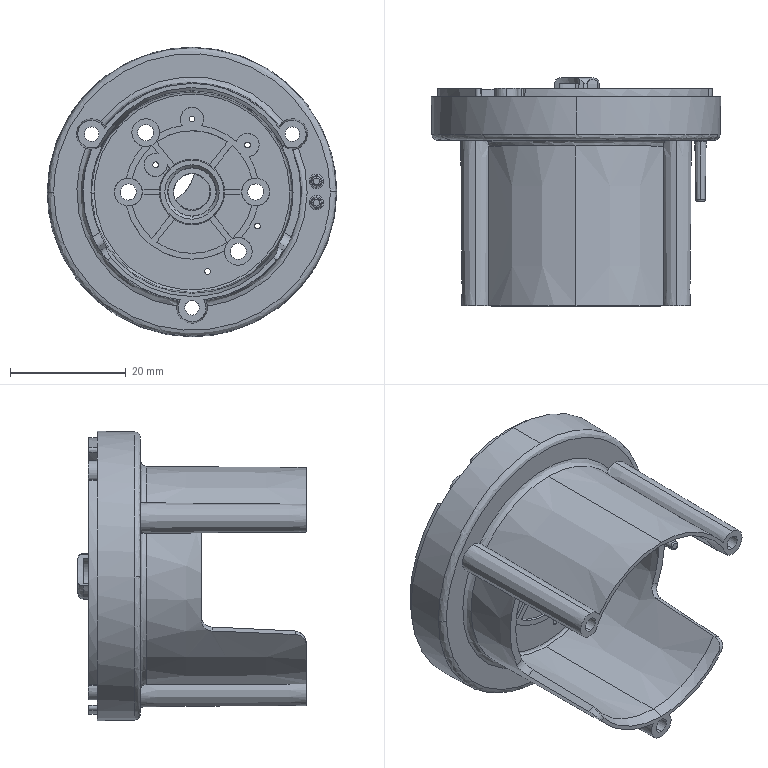Part | SolidWorks | features BaseBody 1 | 1 solid | 269 faces | box 50.005 x 39.4 x 50.005 mm | volume 11183 mm3 | cone 108 | cylinder 79 | plane 64 | spline 18 | commonest cylinder face diameters 4 x26 1.95 x10 2.8 x8 4.8 x8 21.2 x8 23.2 x7